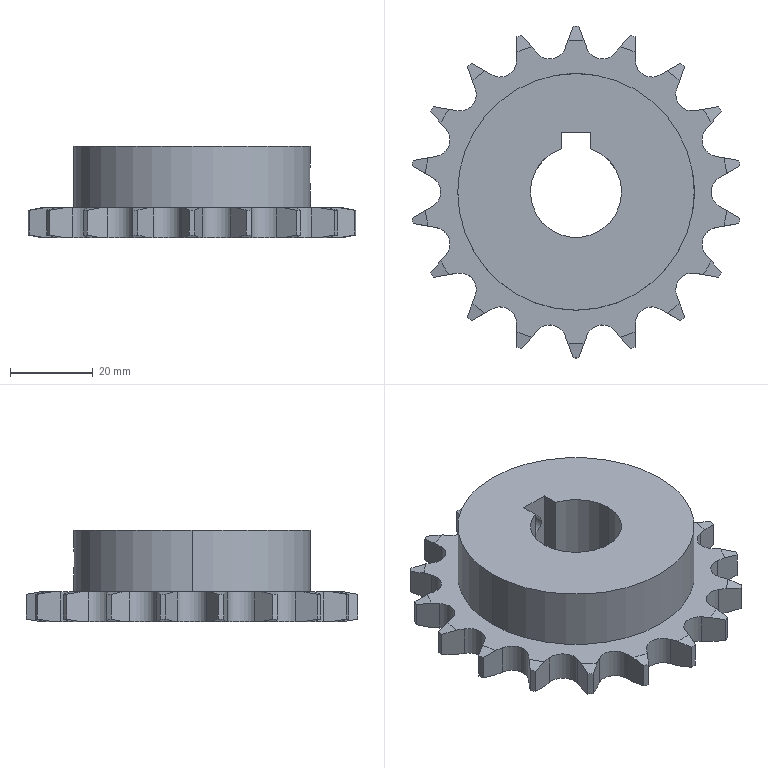Part | SolidWorks | features BaseBody 1 | 1 solid | 129 faces | box 79.007 x 80 x 22 mm | volume 56418 mm3 | cylinder 50 | plane 43 | cone 36 | commonest cylinder face diameters 7.95 x23 80 x18 5 x4 22 x3 57 x2